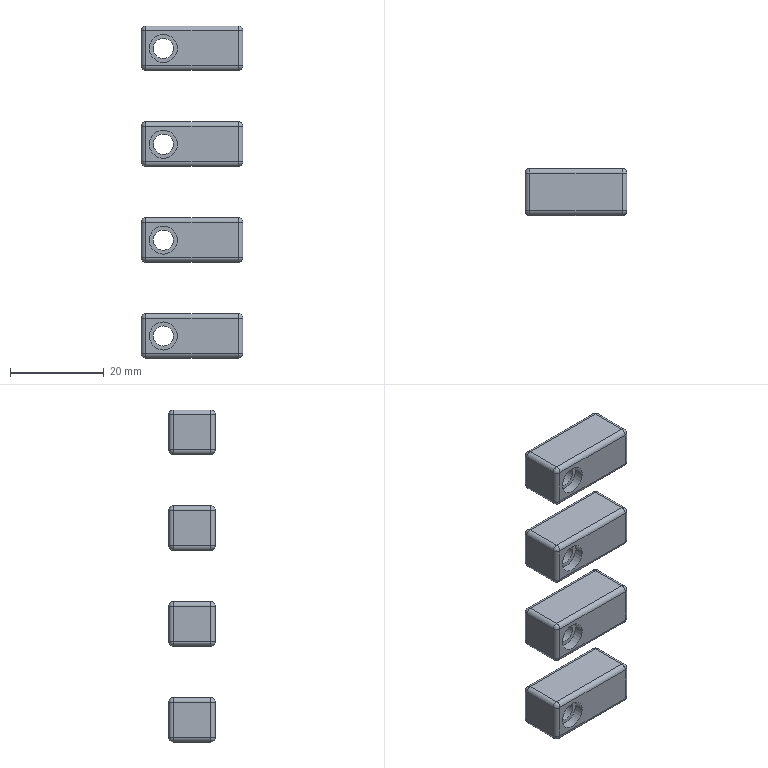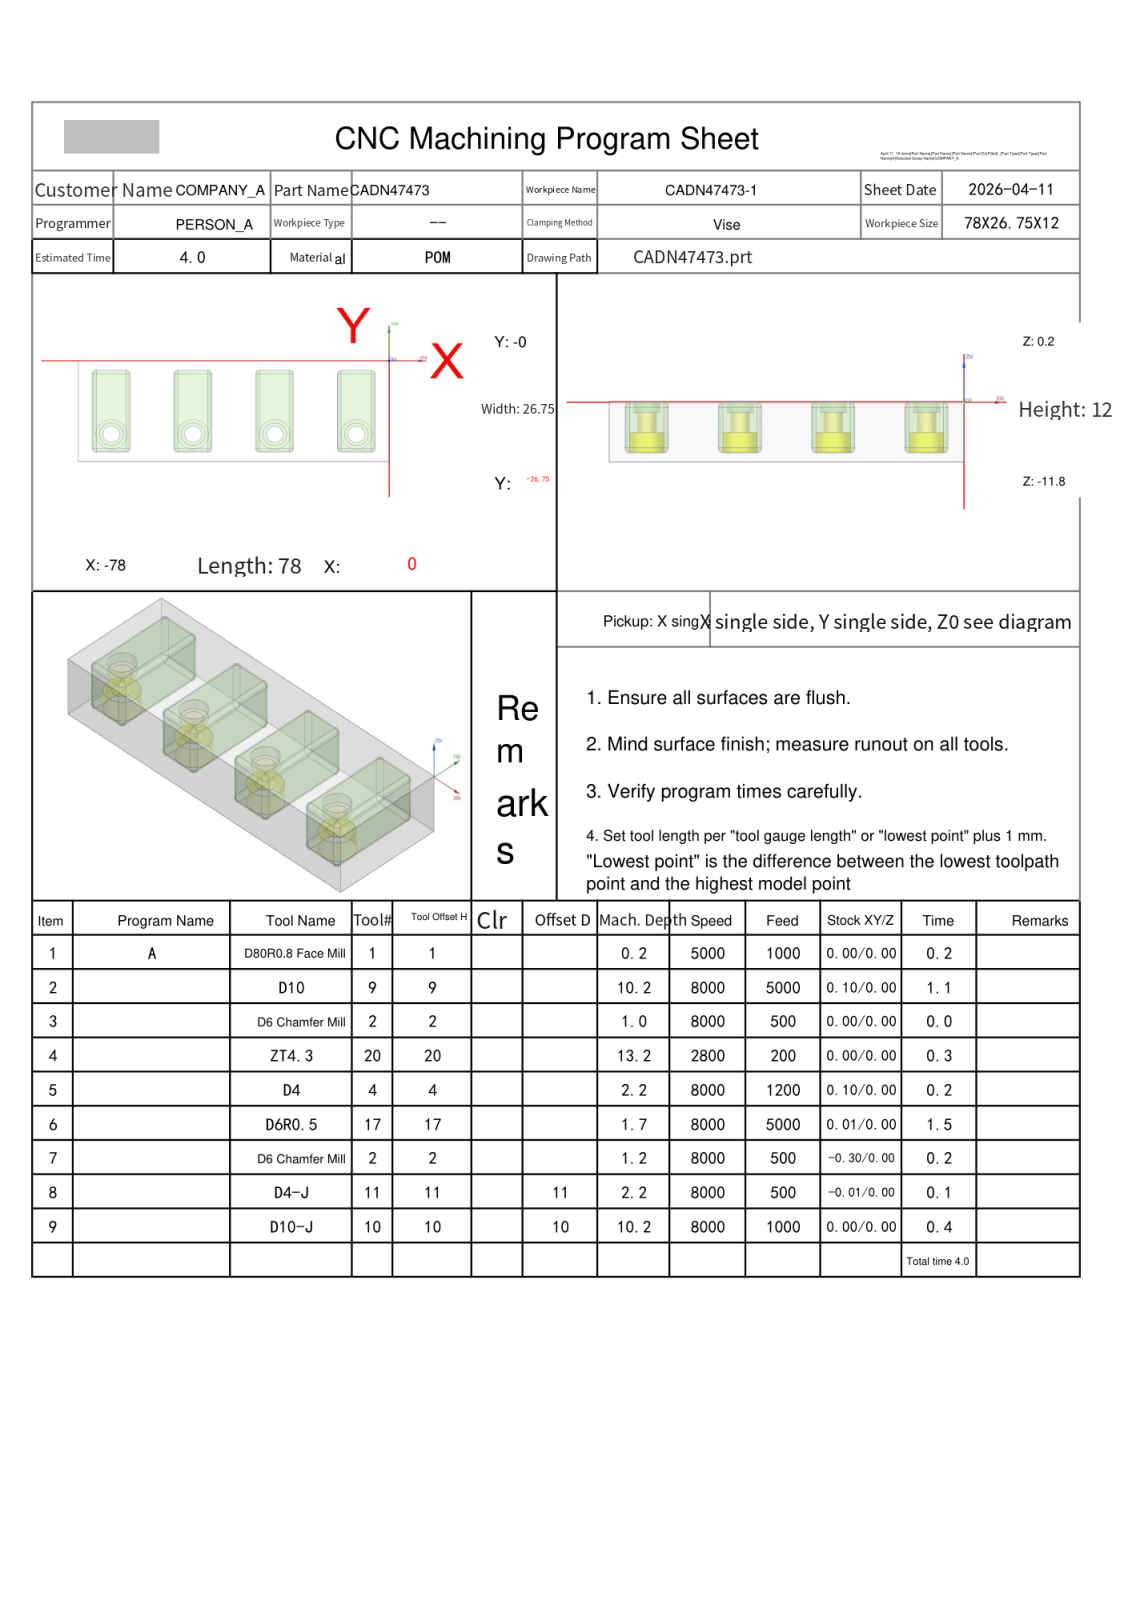NC program | NX | posted by the shop | part box 21.75 x 10 x 71 mm
Lines 1 to 680 of 15665:
%
O0001
(Machine time: 5.91 MIN)
(===Total Tool:8===)
(T1=D80R0.8 Face Mill D=80.  R=0.8  D-  H01 Z=0.    )
(T9=D10     D=10.  R=0.   D-  H09 Z=-10.  )
(T2=D6 Chamfer Mill   D=6.   R=0.   D-  H02 Z=-1.   )
(T20=ZT4.3  D=4.3  DR_a=118 D-  H20 Z=-13.  )
(T4=D4      D=4.   R=0.   D-  H04 Z=-2.   )
(T17=D6R0.5 D=6.   R=0.5  D-  H17 Z=-1.5  )
(T11=D4-J   D=4.   R=0.   D11 H11 Z=-2.   )
(T10=D10-J  D=10.  R=0.   D10 H10 Z=-10.  )
G80 G90 G17 G49 G40
G91 G28 Z0
M01
N1 T01 M06
(D80R0.8 Face Mill  D=80. R=0.8 H=01 ce=0.00 di=0.00)
G00 G90 G54 X41.5 Y-13.375 M03 S5000
G43 H01 Z20.
M08
Z2.
G01 Z0.0 F1000.
X36.5
X-114.5
X-119.5
Z2.
G00 Z20.
G91 G28 Z0.0
M05
M09
G91 G28 Z0.0
M01
N2 T09 M06
(D10  D=10. R=0. H=09 ce=0.10 di=0.00)
G00 G90 G54 X-79.6 Y-13.375 M03 S8000
G43 H09 Z20.
M08
Z.5
G01 Y-3.5 Z.42 F5000.
G02 X-73.5 Y2.6 Z.343 I6.1 J0.0
G01 X-66. Z.282
G02 X-59.9 Y-3.5 Z.205 I0.0 J-6.1
G01 Y-23.25 Z.045
G02 X-66. Y-29.35 Z-.032 I-6.1 J0.0
G01 X-73.5 Z-.093
G02 X-79.6 Y-23.25 Z-.17 I0.0 J6.1
G01 Y-3.5 Z-.33
G02 X-73.5 Y2.6 Z-.407 I6.1 J0.0
G01 X-66. Z-.468
G02 X-59.9 Y-3.5 Z-.545 I0.0 J-6.1
G01 Y-23.25 Z-.705
G02 X-66. Y-29.35 Z-.782 I-6.1 J0.0
G01 X-73.5 Z-.843
G02 X-79.6 Y-23.25 Z-.92 I0.0 J6.1
G01 Y-3.5 Z-1.08
G02 X-73.5 Y2.6 Z-1.157 I6.1 J0.0
G01 X-66. Z-1.218
G02 X-59.9 Y-3.5 Z-1.295 I0.0 J-6.1
G01 Y-23.25 Z-1.455
G02 X-66. Y-29.35 Z-1.532 I-6.1 J0.0
G01 X-73.5 Z-1.593
G02 X-79.6 Y-23.25 Z-1.67 I0.0 J6.1
G01 Y-3.5 Z-1.83
G02 X-73.5 Y2.6 Z-1.907 I6.1 J0.0
G01 X-66. Z-1.968
G02 X-59.9 Y-3.5 Z-2.045 I0.0 J-6.1
G01 Y-23.25 Z-2.205
G02 X-66. Y-29.35 Z-2.282 I-6.1 J0.0
G01 X-73.5 Z-2.343
G02 X-79.6 Y-23.25 Z-2.42 I0.0 J6.1
G01 Y-3.5 Z-2.58
G02 X-73.5 Y2.6 Z-2.657 I6.1 J0.0
G01 X-66. Z-2.718
G02 X-59.9 Y-3.5 Z-2.795 I0.0 J-6.1
G01 Y-23.25 Z-2.955
G02 X-66. Y-29.35 Z-3.032 I-6.1 J0.0
G01 X-73.5 Z-3.093
G02 X-79.6 Y-23.25 Z-3.17 I0.0 J6.1
G01 Y-3.5 Z-3.33
G02 X-73.5 Y2.6 Z-3.407 I6.1 J0.0
G01 X-66. Z-3.468
G02 X-59.9 Y-3.5 Z-3.545 I0.0 J-6.1
G01 Y-23.25 Z-3.705
G02 X-66. Y-29.35 Z-3.782 I-6.1 J0.0
G01 X-73.5 Z-3.843
G02 X-79.6 Y-23.25 Z-3.92 I0.0 J6.1
G01 Y-3.5 Z-4.08
G02 X-73.5 Y2.6 Z-4.157 I6.1 J0.0
G01 X-66. Z-4.218
G02 X-59.9 Y-3.5 Z-4.295 I0.0 J-6.1
G01 Y-23.25 Z-4.455
G02 X-66. Y-29.35 Z-4.532 I-6.1 J0.0
G01 X-73.5 Z-4.593
G02 X-79.6 Y-23.25 Z-4.67 I0.0 J6.1
G01 Y-3.5 Z-4.83
G02 X-73.5 Y2.6 Z-4.907 I6.1 J0.0
G01 X-66. Z-4.968
G02 X-59.9 Y-3.5 Z-5.045 I0.0 J-6.1
G01 Y-23.25 Z-5.205
G02 X-66. Y-29.35 Z-5.282 I-6.1 J0.0
G01 X-73.5 Z-5.343
G02 X-79.6 Y-23.25 Z-5.42 I0.0 J6.1
G01 Y-3.5 Z-5.58
G02 X-73.5 Y2.6 Z-5.657 I6.1 J0.0
G01 X-66. Z-5.718
G02 X-59.9 Y-3.5 Z-5.795 I0.0 J-6.1
G01 Y-23.25 Z-5.955
G02 X-66. Y-29.35 Z-6.032 I-6.1 J0.0
G01 X-73.5 Z-6.093
G02 X-79.6 Y-23.25 Z-6.17 I0.0 J6.1
G01 Y-3.5 Z-6.33
G02 X-73.5 Y2.6 Z-6.407 I6.1 J0.0
G01 X-66. Z-6.468
G02 X-59.9 Y-3.5 Z-6.545 I0.0 J-6.1
G01 Y-23.25 Z-6.705
G02 X-66. Y-29.35 Z-6.782 I-6.1 J0.0
G01 X-73.5 Z-6.843
G02 X-79.6 Y-23.25 Z-6.92 I0.0 J6.1
G01 Y-3.5 Z-7.08
G02 X-73.5 Y2.6 Z-7.157 I6.1 J0.0
G01 X-66. Z-7.218
G02 X-59.9 Y-3.5 Z-7.295 I0.0 J-6.1
G01 Y-23.25 Z-7.455
G02 X-66. Y-29.35 Z-7.532 I-6.1 J0.0
G01 X-73.5 Z-7.593
G02 X-79.6 Y-23.25 Z-7.67 I0.0 J6.1
G01 Y-3.5 Z-7.83
G02 X-73.5 Y2.6 Z-7.907 I6.1 J0.0
G01 X-66. Z-7.968
G02 X-59.9 Y-3.5 Z-8.045 I0.0 J-6.1
G01 Y-23.25 Z-8.205
G02 X-66. Y-29.35 Z-8.282 I-6.1 J0.0
G01 X-73.5 Z-8.343
G02 X-79.6 Y-23.25 Z-8.42 I0.0 J6.1
G01 Y-3.5 Z-8.58
G02 X-73.5 Y2.6 Z-8.657 I6.1 J0.0
G01 X-66. Z-8.718
G02 X-59.9 Y-3.5 Z-8.795 I0.0 J-6.1
G01 Y-23.25 Z-8.955
G02 X-66. Y-29.35 Z-9.032 I-6.1 J0.0
G01 X-73.5 Z-9.093
G02 X-79.6 Y-23.25 Z-9.17 I0.0 J6.1
G01 Y-3.5 Z-9.33
G02 X-73.5 Y2.6 Z-9.407 I6.1 J0.0
G01 X-66. Z-9.468
G02 X-59.9 Y-3.5 Z-9.545 I0.0 J-6.1
G01 Y-23.25 Z-9.705
G02 X-66. Y-29.35 Z-9.782 I-6.1 J0.0
G01 X-73.5 Z-9.843
G02 X-79.6 Y-23.25 Z-9.92 I0.0 J6.1
G01 Y-13.375 Z-10.
Y-3.5
G02 X-73.5 Y2.6 I6.1 J0.0
G01 X-66.
G02 X-59.9 Y-3.5 I0.0 J-6.1
G01 Y-23.25
G02 X-66. Y-29.35 I-6.1 J0.0
G01 X-73.5
G02 X-79.6 Y-23.25 I0.0 J6.1
G01 Y-13.375
Y-12.875
Z-9.
G00 Z20.
X-59.1 Y-13.375
Z.5
G01 Y-3.5 Z.42
G02 X-53. Y2.6 Z.343 I6.1 J0.0
G01 X-45.5 Z.282
G02 X-39.4 Y-3.5 Z.205 I0.0 J-6.1
G01 Y-23.25 Z.045
G02 X-45.5 Y-29.35 Z-.032 I-6.1 J0.0
G01 X-53. Z-.093
G02 X-59.1 Y-23.25 Z-.17 I0.0 J6.1
G01 Y-3.5 Z-.33
G02 X-53. Y2.6 Z-.407 I6.1 J0.0
G01 X-45.5 Z-.468
G02 X-39.4 Y-3.5 Z-.545 I0.0 J-6.1
G01 Y-23.25 Z-.705
G02 X-45.5 Y-29.35 Z-.782 I-6.1 J0.0
G01 X-53. Z-.843
G02 X-59.1 Y-23.25 Z-.92 I0.0 J6.1
G01 Y-3.5 Z-1.08
G02 X-53. Y2.6 Z-1.157 I6.1 J0.0
G01 X-45.5 Z-1.218
G02 X-39.4 Y-3.5 Z-1.295 I0.0 J-6.1
G01 Y-23.25 Z-1.455
G02 X-45.5 Y-29.35 Z-1.532 I-6.1 J0.0
G01 X-53. Z-1.593
G02 X-59.1 Y-23.25 Z-1.67 I0.0 J6.1
G01 Y-3.5 Z-1.83
G02 X-53. Y2.6 Z-1.907 I6.1 J0.0
G01 X-45.5 Z-1.968
G02 X-39.4 Y-3.5 Z-2.045 I0.0 J-6.1
G01 Y-23.25 Z-2.205
G02 X-45.5 Y-29.35 Z-2.282 I-6.1 J0.0
G01 X-53. Z-2.343
G02 X-59.1 Y-23.25 Z-2.42 I0.0 J6.1
G01 Y-3.5 Z-2.58
G02 X-53. Y2.6 Z-2.657 I6.1 J0.0
G01 X-45.5 Z-2.718
G02 X-39.4 Y-3.5 Z-2.795 I0.0 J-6.1
G01 Y-23.25 Z-2.955
G02 X-45.5 Y-29.35 Z-3.032 I-6.1 J0.0
G01 X-53. Z-3.093
G02 X-59.1 Y-23.25 Z-3.17 I0.0 J6.1
G01 Y-3.5 Z-3.33
G02 X-53. Y2.6 Z-3.407 I6.1 J0.0
G01 X-45.5 Z-3.468
G02 X-39.4 Y-3.5 Z-3.545 I0.0 J-6.1
G01 Y-23.25 Z-3.705
G02 X-45.5 Y-29.35 Z-3.782 I-6.1 J0.0
G01 X-53. Z-3.843
G02 X-59.1 Y-23.25 Z-3.92 I0.0 J6.1
G01 Y-3.5 Z-4.08
G02 X-53. Y2.6 Z-4.157 I6.1 J0.0
G01 X-45.5 Z-4.218
G02 X-39.4 Y-3.5 Z-4.295 I0.0 J-6.1
G01 Y-23.25 Z-4.455
G02 X-45.5 Y-29.35 Z-4.532 I-6.1 J0.0
G01 X-53. Z-4.593
G02 X-59.1 Y-23.25 Z-4.67 I0.0 J6.1
G01 Y-3.5 Z-4.83
G02 X-53. Y2.6 Z-4.907 I6.1 J0.0
G01 X-45.5 Z-4.968
G02 X-39.4 Y-3.5 Z-5.045 I0.0 J-6.1
G01 Y-23.25 Z-5.205
G02 X-45.5 Y-29.35 Z-5.282 I-6.1 J0.0
G01 X-53. Z-5.343
G02 X-59.1 Y-23.25 Z-5.42 I0.0 J6.1
G01 Y-3.5 Z-5.58
G02 X-53. Y2.6 Z-5.657 I6.1 J0.0
G01 X-45.5 Z-5.718
G02 X-39.4 Y-3.5 Z-5.795 I0.0 J-6.1
G01 Y-23.25 Z-5.955
G02 X-45.5 Y-29.35 Z-6.032 I-6.1 J0.0
G01 X-53. Z-6.093
G02 X-59.1 Y-23.25 Z-6.17 I0.0 J6.1
G01 Y-3.5 Z-6.33
G02 X-53. Y2.6 Z-6.407 I6.1 J0.0
G01 X-45.5 Z-6.468
G02 X-39.4 Y-3.5 Z-6.545 I0.0 J-6.1
G01 Y-23.25 Z-6.705
G02 X-45.5 Y-29.35 Z-6.782 I-6.1 J0.0
G01 X-53. Z-6.843
G02 X-59.1 Y-23.25 Z-6.92 I0.0 J6.1
G01 Y-3.5 Z-7.08
G02 X-53. Y2.6 Z-7.157 I6.1 J0.0
G01 X-45.5 Z-7.218
G02 X-39.4 Y-3.5 Z-7.295 I0.0 J-6.1
G01 Y-23.25 Z-7.455
G02 X-45.5 Y-29.35 Z-7.532 I-6.1 J0.0
G01 X-53. Z-7.593
G02 X-59.1 Y-23.25 Z-7.67 I0.0 J6.1
G01 Y-3.5 Z-7.83
G02 X-53. Y2.6 Z-7.907 I6.1 J0.0
G01 X-45.5 Z-7.968
G02 X-39.4 Y-3.5 Z-8.045 I0.0 J-6.1
G01 Y-23.25 Z-8.205
G02 X-45.5 Y-29.35 Z-8.282 I-6.1 J0.0
G01 X-53. Z-8.343
G02 X-59.1 Y-23.25 Z-8.42 I0.0 J6.1
G01 Y-3.5 Z-8.58
G02 X-53. Y2.6 Z-8.657 I6.1 J0.0
G01 X-45.5 Z-8.718
G02 X-39.4 Y-3.5 Z-8.795 I0.0 J-6.1
G01 Y-23.25 Z-8.955
G02 X-45.5 Y-29.35 Z-9.032 I-6.1 J0.0
G01 X-53. Z-9.093
G02 X-59.1 Y-23.25 Z-9.17 I0.0 J6.1
G01 Y-3.5 Z-9.33
G02 X-53. Y2.6 Z-9.407 I6.1 J0.0
G01 X-45.5 Z-9.468
G02 X-39.4 Y-3.5 Z-9.545 I0.0 J-6.1
G01 Y-23.25 Z-9.705
G02 X-45.5 Y-29.35 Z-9.782 I-6.1 J0.0
G01 X-53. Z-9.843
G02 X-59.1 Y-23.25 Z-9.92 I0.0 J6.1
G01 Y-13.375 Z-10.
Y-3.5
G02 X-53. Y2.6 I6.1 J0.0
G01 X-45.5
G02 X-39.4 Y-3.5 I0.0 J-6.1
G01 Y-23.25
G02 X-45.5 Y-29.35 I-6.1 J0.0
G01 X-53.
G02 X-59.1 Y-23.25 I0.0 J6.1
G01 Y-13.375
Y-12.875
Z-9.
G00 Z20.
X-38.6 Y-13.375
Z.5
G01 Y-3.5 Z.42
G02 X-32.5 Y2.6 Z.343 I6.1 J0.0
G01 X-25. Z.282
G02 X-18.9 Y-3.5 Z.205 I0.0 J-6.1
G01 Y-23.25 Z.045
G02 X-25. Y-29.35 Z-.032 I-6.1 J0.0
G01 X-32.5 Z-.093
G02 X-38.6 Y-23.25 Z-.17 I0.0 J6.1
G01 Y-3.5 Z-.33
G02 X-32.5 Y2.6 Z-.407 I6.1 J0.0
G01 X-25. Z-.468
G02 X-18.9 Y-3.5 Z-.545 I0.0 J-6.1
G01 Y-23.25 Z-.705
G02 X-25. Y-29.35 Z-.782 I-6.1 J0.0
G01 X-32.5 Z-.843
G02 X-38.6 Y-23.25 Z-.92 I0.0 J6.1
G01 Y-3.5 Z-1.08
G02 X-32.5 Y2.6 Z-1.157 I6.1 J0.0
G01 X-25. Z-1.218
G02 X-18.9 Y-3.5 Z-1.295 I0.0 J-6.1
G01 Y-23.25 Z-1.455
G02 X-25. Y-29.35 Z-1.532 I-6.1 J0.0
G01 X-32.5 Z-1.593
G02 X-38.6 Y-23.25 Z-1.67 I0.0 J6.1
G01 Y-3.5 Z-1.83
G02 X-32.5 Y2.6 Z-1.907 I6.1 J0.0
G01 X-25. Z-1.968
G02 X-18.9 Y-3.5 Z-2.045 I0.0 J-6.1
G01 Y-23.25 Z-2.205
G02 X-25. Y-29.35 Z-2.282 I-6.1 J0.0
G01 X-32.5 Z-2.343
G02 X-38.6 Y-23.25 Z-2.42 I0.0 J6.1
G01 Y-3.5 Z-2.58
G02 X-32.5 Y2.6 Z-2.657 I6.1 J0.0
G01 X-25. Z-2.718
G02 X-18.9 Y-3.5 Z-2.795 I0.0 J-6.1
G01 Y-23.25 Z-2.955
G02 X-25. Y-29.35 Z-3.032 I-6.1 J0.0
G01 X-32.5 Z-3.093
G02 X-38.6 Y-23.25 Z-3.17 I0.0 J6.1
G01 Y-3.5 Z-3.33
G02 X-32.5 Y2.6 Z-3.407 I6.1 J0.0
G01 X-25. Z-3.468
G02 X-18.9 Y-3.5 Z-3.545 I0.0 J-6.1
G01 Y-23.25 Z-3.705
G02 X-25. Y-29.35 Z-3.782 I-6.1 J0.0
G01 X-32.5 Z-3.843
G02 X-38.6 Y-23.25 Z-3.92 I0.0 J6.1
G01 Y-3.5 Z-4.08
G02 X-32.5 Y2.6 Z-4.157 I6.1 J0.0
G01 X-25. Z-4.218
G02 X-18.9 Y-3.5 Z-4.295 I0.0 J-6.1
G01 Y-23.25 Z-4.455
G02 X-25. Y-29.35 Z-4.532 I-6.1 J0.0
G01 X-32.5 Z-4.593
G02 X-38.6 Y-23.25 Z-4.67 I0.0 J6.1
G01 Y-3.5 Z-4.83
G02 X-32.5 Y2.6 Z-4.907 I6.1 J0.0
G01 X-25. Z-4.968
G02 X-18.9 Y-3.5 Z-5.045 I0.0 J-6.1
G01 Y-23.25 Z-5.205
G02 X-25. Y-29.35 Z-5.282 I-6.1 J0.0
G01 X-32.5 Z-5.343
G02 X-38.6 Y-23.25 Z-5.42 I0.0 J6.1
G01 Y-3.5 Z-5.58
G02 X-32.5 Y2.6 Z-5.657 I6.1 J0.0
G01 X-25. Z-5.718
G02 X-18.9 Y-3.5 Z-5.795 I0.0 J-6.1
G01 Y-23.25 Z-5.955
G02 X-25. Y-29.35 Z-6.032 I-6.1 J0.0
G01 X-32.5 Z-6.093
G02 X-38.6 Y-23.25 Z-6.17 I0.0 J6.1
G01 Y-3.5 Z-6.33
G02 X-32.5 Y2.6 Z-6.407 I6.1 J0.0
G01 X-25. Z-6.468
G02 X-18.9 Y-3.5 Z-6.545 I0.0 J-6.1
G01 Y-23.25 Z-6.705
G02 X-25. Y-29.35 Z-6.782 I-6.1 J0.0
G01 X-32.5 Z-6.843
G02 X-38.6 Y-23.25 Z-6.92 I0.0 J6.1
G01 Y-3.5 Z-7.08
G02 X-32.5 Y2.6 Z-7.157 I6.1 J0.0
G01 X-25. Z-7.218
G02 X-18.9 Y-3.5 Z-7.295 I0.0 J-6.1
G01 Y-23.25 Z-7.455
G02 X-25. Y-29.35 Z-7.532 I-6.1 J0.0
G01 X-32.5 Z-7.593
G02 X-38.6 Y-23.25 Z-7.67 I0.0 J6.1
G01 Y-3.5 Z-7.83
G02 X-32.5 Y2.6 Z-7.907 I6.1 J0.0
G01 X-25. Z-7.968
G02 X-18.9 Y-3.5 Z-8.045 I0.0 J-6.1
G01 Y-23.25 Z-8.205
G02 X-25. Y-29.35 Z-8.282 I-6.1 J0.0
G01 X-32.5 Z-8.343
G02 X-38.6 Y-23.25 Z-8.42 I0.0 J6.1
G01 Y-3.5 Z-8.58
G02 X-32.5 Y2.6 Z-8.657 I6.1 J0.0
G01 X-25. Z-8.718
G02 X-18.9 Y-3.5 Z-8.795 I0.0 J-6.1
G01 Y-23.25 Z-8.955
G02 X-25. Y-29.35 Z-9.032 I-6.1 J0.0
G01 X-32.5 Z-9.093
G02 X-38.6 Y-23.25 Z-9.17 I0.0 J6.1
G01 Y-3.5 Z-9.33
G02 X-32.5 Y2.6 Z-9.407 I6.1 J0.0
G01 X-25. Z-9.468
G02 X-18.9 Y-3.5 Z-9.545 I0.0 J-6.1
G01 Y-23.25 Z-9.705
G02 X-25. Y-29.35 Z-9.782 I-6.1 J0.0
G01 X-32.5 Z-9.843
G02 X-38.6 Y-23.25 Z-9.92 I0.0 J6.1
G01 Y-13.375 Z-10.
Y-3.5
G02 X-32.5 Y2.6 I6.1 J0.0
G01 X-25.
G02 X-18.9 Y-3.5 I0.0 J-6.1
G01 Y-23.25
G02 X-25. Y-29.35 I-6.1 J0.0
G01 X-32.5
G02 X-38.6 Y-23.25 I0.0 J6.1
G01 Y-13.375
Y-12.875
Z-9.
G00 Z20.
X1.6 Y-13.375
Z.5
G01 Y-23.25 Z.42
G02 X-4.5 Y-29.35 Z.343 I-6.1 J0.0
G01 X-12. Z.282
G02 X-18.1 Y-23.25 Z.205 I0.0 J6.1
G01 Y-3.5 Z.045
G02 X-12. Y2.6 Z-.032 I6.1 J0.0
G01 X-4.5 Z-.093
G02 X1.6 Y-3.5 Z-.17 I0.0 J-6.1
G01 Y-23.25 Z-.33
G02 X-4.5 Y-29.35 Z-.407 I-6.1 J0.0
G01 X-12. Z-.468
G02 X-18.1 Y-23.25 Z-.545 I0.0 J6.1
G01 Y-3.5 Z-.705
G02 X-12. Y2.6 Z-.782 I6.1 J0.0
G01 X-4.5 Z-.843
G02 X1.6 Y-3.5 Z-.92 I0.0 J-6.1
G01 Y-23.25 Z-1.08
G02 X-4.5 Y-29.35 Z-1.157 I-6.1 J0.0
G01 X-12. Z-1.218
G02 X-18.1 Y-23.25 Z-1.295 I0.0 J6.1
G01 Y-3.5 Z-1.455
G02 X-12. Y2.6 Z-1.532 I6.1 J0.0
G01 X-4.5 Z-1.593
G02 X1.6 Y-3.5 Z-1.67 I0.0 J-6.1
G01 Y-23.25 Z-1.83
G02 X-4.5 Y-29.35 Z-1.907 I-6.1 J0.0
G01 X-12. Z-1.968
G02 X-18.1 Y-23.25 Z-2.045 I0.0 J6.1
G01 Y-3.5 Z-2.205
G02 X-12. Y2.6 Z-2.282 I6.1 J0.0
G01 X-4.5 Z-2.343
G02 X1.6 Y-3.5 Z-2.42 I0.0 J-6.1
G01 Y-23.25 Z-2.58
G02 X-4.5 Y-29.35 Z-2.657 I-6.1 J0.0
G01 X-12. Z-2.718
G02 X-18.1 Y-23.25 Z-2.795 I0.0 J6.1
G01 Y-3.5 Z-2.955
G02 X-12. Y2.6 Z-3.032 I6.1 J0.0
G01 X-4.5 Z-3.093
G02 X1.6 Y-3.5 Z-3.17 I0.0 J-6.1
G01 Y-23.25 Z-3.33
G02 X-4.5 Y-29.35 Z-3.407 I-6.1 J0.0
G01 X-12. Z-3.468
G02 X-18.1 Y-23.25 Z-3.545 I0.0 J6.1
G01 Y-3.5 Z-3.705
G02 X-12. Y2.6 Z-3.782 I6.1 J0.0
G01 X-4.5 Z-3.843
G02 X1.6 Y-3.5 Z-3.92 I0.0 J-6.1
G01 Y-23.25 Z-4.08
G02 X-4.5 Y-29.35 Z-4.157 I-6.1 J0.0
G01 X-12. Z-4.218
G02 X-18.1 Y-23.25 Z-4.295 I0.0 J6.1
G01 Y-3.5 Z-4.455
G02 X-12. Y2.6 Z-4.532 I6.1 J0.0
G01 X-4.5 Z-4.593
G02 X1.6 Y-3.5 Z-4.67 I0.0 J-6.1
G01 Y-23.25 Z-4.83
G02 X-4.5 Y-29.35 Z-4.907 I-6.1 J0.0
G01 X-12. Z-4.968
G02 X-18.1 Y-23.25 Z-5.045 I0.0 J6.1
G01 Y-3.5 Z-5.205
G02 X-12. Y2.6 Z-5.282 I6.1 J0.0
G01 X-4.5 Z-5.343
G02 X1.6 Y-3.5 Z-5.42 I0.0 J-6.1
G01 Y-23.25 Z-5.58
G02 X-4.5 Y-29.35 Z-5.657 I-6.1 J0.0
G01 X-12. Z-5.718
G02 X-18.1 Y-23.25 Z-5.795 I0.0 J6.1
G01 Y-3.5 Z-5.955
G02 X-12. Y2.6 Z-6.032 I6.1 J0.0
G01 X-4.5 Z-6.093
G02 X1.6 Y-3.5 Z-6.17 I0.0 J-6.1
G01 Y-23.25 Z-6.33
G02 X-4.5 Y-29.35 Z-6.407 I-6.1 J0.0
G01 X-12. Z-6.468
G02 X-18.1 Y-23.25 Z-6.545 I0.0 J6.1
G01 Y-3.5 Z-6.705
G02 X-12. Y2.6 Z-6.782 I6.1 J0.0
G01 X-4.5 Z-6.843
G02 X1.6 Y-3.5 Z-6.92 I0.0 J-6.1
G01 Y-23.25 Z-7.08
G02 X-4.5 Y-29.35 Z-7.157 I-6.1 J0.0
G01 X-12. Z-7.218
G02 X-18.1 Y-23.25 Z-7.295 I0.0 J6.1
G01 Y-3.5 Z-7.455
G02 X-12. Y2.6 Z-7.532 I6.1 J0.0
G01 X-4.5 Z-7.593
G02 X1.6 Y-3.5 Z-7.67 I0.0 J-6.1
G01 Y-23.25 Z-7.83
G02 X-4.5 Y-29.35 Z-7.907 I-6.1 J0.0
G01 X-12. Z-7.968
G02 X-18.1 Y-23.25 Z-8.045 I0.0 J6.1
G01 Y-3.5 Z-8.205
G02 X-12. Y2.6 Z-8.282 I6.1 J0.0
G01 X-4.5 Z-8.343
G02 X1.6 Y-3.5 Z-8.42 I0.0 J-6.1
G01 Y-23.25 Z-8.58
G02 X-4.5 Y-29.35 Z-8.657 I-6.1 J0.0
G01 X-12. Z-8.718
G02 X-18.1 Y-23.25 Z-8.795 I0.0 J6.1
G01 Y-3.5 Z-8.955
G02 X-12. Y2.6 Z-9.032 I6.1 J0.0
G01 X-4.5 Z-9.093
G02 X1.6 Y-3.5 Z-9.17 I0.0 J-6.1
G01 Y-23.25 Z-9.33
G02 X-4.5 Y-29.35 Z-9.407 I-6.1 J0.0
G01 X-12. Z-9.468
G02 X-18.1 Y-23.25 Z-9.545 I0.0 J6.1
G01 Y-3.5 Z-9.705
G02 X-12. Y2.6 Z-9.782 I6.1 J0.0
G01 X-4.5 Z-9.843
G02 X1.6 Y-3.5 Z-9.92 I0.0 J-6.1
G01 Y-13.375 Z-10.
Y-23.25
G02 X-4.5 Y-29.35 I-6.1 J0.0
G01 X-12.
G02 X-18.1 Y-23.25 I0.0 J6.1
G01 Y-3.5
G02 X-12. Y2.6 I6.1 J0.0
G01 X-4.5
G02 X1.6 Y-3.5 I0.0 J-6.1
G01 Y-13.375
Y-13.875
Z-9.
G00 Z20.
G91 G28 Z0.0
M05
M09
G91 G28 Z0.0
M01
N3 T02 M06
(D6 Chamfer Mill  D=6. R=0. H=02 ce=0.00 di=0.00)
G00 G90 G54 X-69.704 Y-19.5 M03 S8000
G43 H02 Z20.
M08
G98 G81 X-69.704 Y-19.5 Z-.8 R1. F500.
X-49.204
X-28.704
X-8.204
G80
G00 Z20.
G91 G28 Z0.0
M05
M09
G91 G28 Z0.0
M01
N4 T20 M06
(ZT4.3 D=4.3 DR_a=118 H=20)
G00 G90 G54 X-69.704 Y-19.5 M03 S2800
G43 H20 Z20.
M08
G98 G83 X-69.704 Y-19.5 Z-13. R1. F200. Q2.
X-49.204
X-28.704
X-8.204
G80
G00 Z20.
G91 G28 Z0.0
M05
M09
G91 G28 Z0.0
M01
N5 T04 M06
(D4  D=4. R=0. H=04 ce=0.10 di=0.00)
G00 G90 G54 X-69.704 Y-19.5 M03 S8000
G43 H04 Z20.
M08
Z.5
G03 X-69.254 Y-19.05 I0.0 J.45 F1200.
X-69.704 Y-18.6 I-.45 J0.0
X-69.704 Y-18.6 Z.2 I0.0 J-.9
X-69.704 Y-18.6 Z-.1 I0.0 J-.9
X-69.704 Y-18.6 Z-.4 I0.0 J-.9
X-69.704 Y-18.6 Z-.7 I0.0 J-.9
X-69.704 Y-18.6 Z-1. I0.0 J-.9
X-69.704 Y-18.6 Z-1.3 I0.0 J-.9
X-69.704 Y-18.6 Z-1.6 I0.0 J-.9
X-69.704 Y-18.6 Z-1.9 I0.0 J-.9
X-70.483 Y-19.95 Z-2. I0.0 J-.9
X-69.704 Y-20.4 I.779 J.45
X-68.804 Y-19.5 I0.0 J.9
X-69.704 Y-18.6 I-.9 J0.0
X-70.604 Y-19.5 I0.0 J-.9
X-70.483 Y-19.95 I.9 J0.0
X-70.094 Y-20.175 I.39 J.225
X-69.644 Y-19.725 I0.0 J.45
X-69.704 Y-19.5 I-.45 J0.0
G00 Z20.
X-49.204
Z.5
G03 X-48.754 Y-19.05 I0.0 J.45
X-49.204 Y-18.6 I-.45 J0.0
X-49.204 Y-18.6 Z.2 I0.0 J-.9
X-49.204 Y-18.6 Z-.1 I0.0 J-.9
X-49.204 Y-18.6 Z-.4 I0.0 J-.9
X-49.204 Y-18.6 Z-.7 I0.0 J-.9
X-49.204 Y-18.6 Z-1. I0.0 J-.9
X-49.204 Y-18.6 Z-1.3 I0.0 J-.9
X-49.204 Y-18.6 Z-1.6 I0.0 J-.9
X-49.204 Y-18.6 Z-1.9 I0.0 J-.9
X-49.983 Y-19.95 Z-2. I0.0 J-.9
X-49.204 Y-20.4 I.779 J.45
X-48.304 Y-19.5 I0.0 J.9
X-49.204 Y-18.6 I-.9 J0.0
X-50.104 Y-19.5 I0.0 J-.9
X-49.983 Y-19.95 I.9 J0.0
X-49.594 Y-20.175 I.39 J.225
X-49.144 Y-19.725 I0.0 J.45
X-49.204 Y-19.5 I-.45 J0.0
G00 Z20.
X-28.704
Z.5
G03 X-28.254 Y-19.05 I0.0 J.45
X-28.704 Y-18.6 I-.45 J0.0
X-28.704 Y-18.6 Z.2 I0.0 J-.9
X-28.704 Y-18.6 Z-.1 I0.0 J-.9
X-28.704 Y-18.6 Z-.4 I0.0 J-.9
X-28.704 Y-18.6 Z-.7 I0.0 J-.9
X-28.704 Y-18.6 Z-1. I0.0 J-.9
X-28.704 Y-18.6 Z-1.3 I0.0 J-.9
X-28.704 Y-18.6 Z-1.6 I0.0 J-.9
X-28.704 Y-18.6 Z-1.9 I0.0 J-.9
X-29.483 Y-19.95 Z-2. I0.0 J-.9
X-28.704 Y-20.4 I.779 J.45
X-27.804 Y-19.5 I0.0 J.9
X-28.704 Y-18.6 I-.9 J0.0
X-29.604 Y-19.5 I0.0 J-.9
X-29.483 Y-19.95 I.9 J0.0
X-29.094 Y-20.175 I.39 J.225
X-28.644 Y-19.725 I0.0 J.45
X-28.704 Y-19.5 I-.45 J0.0
G00 Z20.
X-8.204
Z.5
G03 X-7.754 Y-19.05 I0.0 J.45
X-8.204 Y-18.6 I-.45 J0.0
X-8.204 Y-18.6 Z.2 I0.0 J-.9
X-8.204 Y-18.6 Z-.1 I0.0 J-.9
X-8.204 Y-18.6 Z-.4 I0.0 J-.9
X-8.204 Y-18.6 Z-.7 I0.0 J-.9
X-8.204 Y-18.6 Z-1. I0.0 J-.9
X-8.204 Y-18.6 Z-1.3 I0.0 J-.9
X-8.204 Y-18.6 Z-1.6 I0.0 J-.9
X-8.204 Y-18.6 Z-1.9 I0.0 J-.9
X-8.983 Y-19.95 Z-2. I0.0 J-.9
X-8.204 Y-20.4 I.779 J.45
X-7.304 Y-19.5 I0.0 J.9
X-8.204 Y-18.6 I-.9 J0.0
X-9.104 Y-19.5 I0.0 J-.9
X-8.983 Y-19.95 I.9 J0.0
X-8.594 Y-20.175 I.39 J.225
X-8.144 Y-19.725 I0.0 J.45
X-8.204 Y-19.5 I-.45 J0.0
G00 Z20.
G91 G28 Z0.0
M05
M09
G91 G28 Z0.0
M01